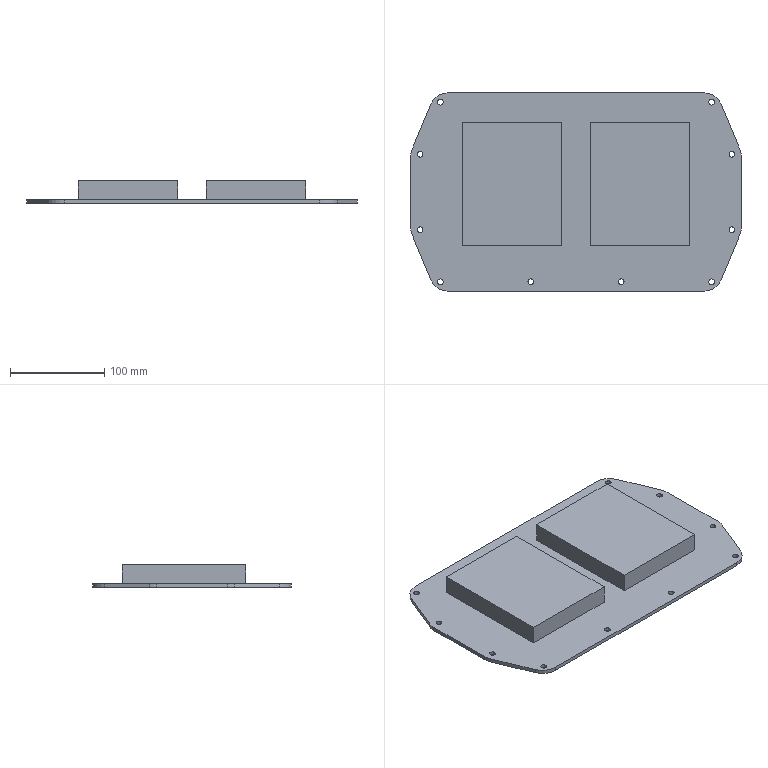Part | SolidWorks | features BaseBody 1 | 1 solid | 48 faces | box 350 x 210 x 24 mm | volume 832302 mm3 | cylinder 28 | plane 20 | commonest cylinder face diameters 6 x20 40 x8